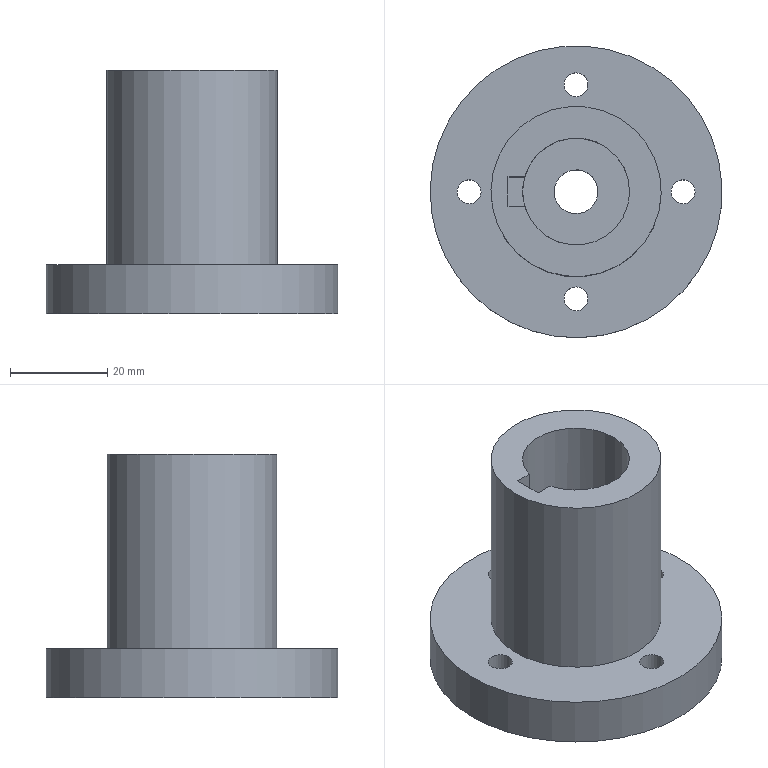Part | STEP file | SN10_010_004_EIXO | 1 solid | 18 faces | box 60 x 60 x 50 mm | volume 51834 mm3 | cylinder 9 | plane 9 | commonest cylinder face diameters 4.917 x4 9 x1 15 x1 22 x1 35 x1 60 x1
STEP:
#1=CARTESIAN_POINT('',(0.,0.,0.));
#2=DIRECTION('',(0.,0.,1.));
#3=DIRECTION('',(1.,0.,0.));
#4=AXIS2_PLACEMENT_3D('',#1,#2,#3);
#5=CARTESIAN_POINT('',(315.286,-1.179,392.5));
#6=VERTEX_POINT('',#5);
#7=CARTESIAN_POINT('',(313.129,0.,392.5));
#8=DIRECTION('',(0.,0.,-1.));
#9=DIRECTION('',(1.,0.,0.));
#10=AXIS2_PLACEMENT_3D('',#7,#8,#9);
#11=CIRCLE('',#10,2.458);
#12=CARTESIAN_POINT('',(313.129,0.,392.4));
#13=DIRECTION('',(0.,0.,-1.));
#14=DIRECTION('',(0.8776,-0.4794,0.));
#15=AXIS2_PLACEMENT_3D('',#12,#13,#14);
#16=CYLINDRICAL_SURFACE('',#15,2.458);
#17=CARTESIAN_POINT('',(-0.5,-0.1));
#18=DIRECTION('',(1.,0.));
#19=VECTOR('',#18,1.);
#20=LINE('',#17,#19);
#21=(GEOMETRIC_REPRESENTATION_CONTEXT(2)PARAMETRIC_REPRESENTATION_CONTEXT()REPRESENTATION_CONTEXT('',''));
#22=DEFINITIONAL_REPRESENTATION('',(#20),#21);
#23=PCURVE('',#16,#22);
#24=CARTESIAN_POINT('',(291.129,17.5,392.5));
#25=DIRECTION('',(0.,0.,1.));
#26=DIRECTION('',(1.,0.,0.));
#27=AXIS2_PLACEMENT_3D('',#24,#25,#26);
#28=PLANE('',#27);
#29=CARTESIAN_POINT('',(24.459,-17.5));
#30=CARTESIAN_POINT('',(24.459,-21.758));
#31=CARTESIAN_POINT('',(20.771,-19.629));
#32=CARTESIAN_POINT('',(17.083,-17.5));
#33=CARTESIAN_POINT('',(20.771,-15.371));
#34=CARTESIAN_POINT('',(24.459,-13.242));
#35=CARTESIAN_POINT('',(24.459,-17.5));
#36=(BOUNDED_CURVE()B_SPLINE_CURVE(2,(#29,#30,#31,#32,#33,#34,#35),.UNSPECIFIED.,.T.,.F.)B_SPLINE_CURVE_WITH_KNOTS((1,2,2,2,2,1),(-2.094,0.,2.094,4.189,6.283,8.378),.UNSPECIFIED.)CURVE()GEOMETRIC_REPRESENTATION_ITEM()RATIONAL_B_SPLINE_CURVE((1.,0.5,1.,0.5,1.,0.5,1.))REPRESENTATION_ITEM(''));
#37=(GEOMETRIC_REPRESENTATION_CONTEXT(2)PARAMETRIC_REPRESENTATION_CONTEXT()REPRESENTATION_CONTEXT('',''));
#38=DEFINITIONAL_REPRESENTATION('',(#36),#37);
#39=PCURVE('',#28,#38);
#40=SURFACE_CURVE('',#11,(#23,#39),.PCURVE_S1.);
#41=EDGE_CURVE('',#6,#6,#40,.T.);
#42=ORIENTED_EDGE('',*,*,#41,.T.);
#43=CARTESIAN_POINT('',(315.286,-1.179,382.5));
#44=VERTEX_POINT('',#43);
#45=CARTESIAN_POINT('',(315.286,-1.179,392.5));
#46=CARTESIAN_POINT('',(315.286,-1.179,382.5));
#47=B_SPLINE_CURVE_WITH_KNOTS('',1,(#45,#46),.UNSPECIFIED.,.F.,.F.,(2,2),(-0.1,9.9),.PIECEWISE_BEZIER_KNOTS.);
#48=CARTESIAN_POINT('',(6.283,0.));
#49=DIRECTION('',(0.,1.));
#50=VECTOR('',#49,1.);
#51=LINE('',#48,#50);
#52=(GEOMETRIC_REPRESENTATION_CONTEXT(2)PARAMETRIC_REPRESENTATION_CONTEXT()REPRESENTATION_CONTEXT('',''));
#53=DEFINITIONAL_REPRESENTATION('',(#51),#52);
#54=PCURVE('',#16,#53);
#55=CARTESIAN_POINT('',(0.,0.));
#56=DIRECTION('',(0.,1.));
#57=VECTOR('',#56,1.);
#58=LINE('',#55,#57);
#59=(GEOMETRIC_REPRESENTATION_CONTEXT(2)PARAMETRIC_REPRESENTATION_CONTEXT()REPRESENTATION_CONTEXT('',''));
#60=DEFINITIONAL_REPRESENTATION('',(#58),#59);
#61=PCURVE('',#16,#60);
#62=SEAM_CURVE('',#47,(#54,#61),.PCURVE_S1.);
#63=EDGE_CURVE('',#6,#44,#62,.T.);
#64=ORIENTED_EDGE('',*,*,#63,.T.);
#65=CARTESIAN_POINT('',(313.129,0.,382.5));
#66=DIRECTION('',(0.,0.,-1.));
#67=DIRECTION('',(1.,0.,0.));
#68=AXIS2_PLACEMENT_3D('',#65,#66,#67);
#69=CIRCLE('',#68,2.458);
#70=CARTESIAN_POINT('',(-0.5,9.9));
#71=DIRECTION('',(1.,0.));
#72=VECTOR('',#71,1.);
#73=LINE('',#70,#72);
#74=(GEOMETRIC_REPRESENTATION_CONTEXT(2)PARAMETRIC_REPRESENTATION_CONTEXT()REPRESENTATION_CONTEXT('',''));
#75=DEFINITIONAL_REPRESENTATION('',(#73),#74);
#76=PCURVE('',#16,#75);
#77=CARTESIAN_POINT('',(291.129,30.,382.5));
#78=DIRECTION('',(0.,0.,1.));
#79=DIRECTION('',(1.,0.,0.));
#80=AXIS2_PLACEMENT_3D('',#77,#78,#79);
#81=PLANE('',#80);
#82=CARTESIAN_POINT('',(24.459,-30.));
#83=CARTESIAN_POINT('',(24.459,-34.258));
#84=CARTESIAN_POINT('',(20.771,-32.129));
#85=CARTESIAN_POINT('',(17.083,-30.));
#86=CARTESIAN_POINT('',(20.771,-27.871));
#87=CARTESIAN_POINT('',(24.459,-25.742));
#88=CARTESIAN_POINT('',(24.459,-30.));
#89=(BOUNDED_CURVE()B_SPLINE_CURVE(2,(#82,#83,#84,#85,#86,#87,#88),.UNSPECIFIED.,.T.,.F.)B_SPLINE_CURVE_WITH_KNOTS((1,2,2,2,2,1),(-2.094,0.,2.094,4.189,6.283,8.378),.UNSPECIFIED.)CURVE()GEOMETRIC_REPRESENTATION_ITEM()RATIONAL_B_SPLINE_CURVE((1.,0.5,1.,0.5,1.,0.5,1.))REPRESENTATION_ITEM(''));
#90=(GEOMETRIC_REPRESENTATION_CONTEXT(2)PARAMETRIC_REPRESENTATION_CONTEXT()REPRESENTATION_CONTEXT('',''));
#91=DEFINITIONAL_REPRESENTATION('',(#89),#90);
#92=PCURVE('',#81,#91);
#93=SURFACE_CURVE('',#69,(#76,#92),.PCURVE_S1.);
#94=EDGE_CURVE('',#44,#44,#93,.T.);
#95=ORIENTED_EDGE('',*,*,#94,.F.);
#96=ORIENTED_EDGE('',*,*,#63,.F.);
#97=EDGE_LOOP('',(#42,#64,#95,#96));
#98=FACE_BOUND('',#97,.F.);
#99=ADVANCED_FACE('',(#98),#16,.F.);
#100=CARTESIAN_POINT('',(305.512,-26.327,382.5));
#101=VERTEX_POINT('',#100);
#102=CARTESIAN_POINT('',(291.129,0.,382.5));
#103=DIRECTION('',(0.,0.,1.));
#104=DIRECTION('',(1.,0.,0.));
#105=AXIS2_PLACEMENT_3D('',#102,#103,#104);
#106=CIRCLE('',#105,30.);
#107=CARTESIAN_POINT('',(291.129,0.,407.5));
#108=DIRECTION('',(0.,0.,1.));
#109=DIRECTION('',(-0.4794,0.8776,0.));
#110=AXIS2_PLACEMENT_3D('',#107,#108,#109);
#111=CYLINDRICAL_SURFACE('',#110,30.);
#112=CARTESIAN_POINT('',(-2.071,-25.));
#113=DIRECTION('',(1.,0.));
#114=VECTOR('',#113,1.);
#115=LINE('',#112,#114);
#116=(GEOMETRIC_REPRESENTATION_CONTEXT(2)PARAMETRIC_REPRESENTATION_CONTEXT()REPRESENTATION_CONTEXT('',''));
#117=DEFINITIONAL_REPRESENTATION('',(#115),#116);
#118=PCURVE('',#111,#117);
#119=CARTESIAN_POINT('',(0.,-30.));
#120=DIRECTION('',(1.,0.));
#121=AXIS2_PLACEMENT_2D('',#119,#120);
#122=CIRCLE('',#121,30.);
#123=(GEOMETRIC_REPRESENTATION_CONTEXT(2)PARAMETRIC_REPRESENTATION_CONTEXT()REPRESENTATION_CONTEXT('',''));
#124=DEFINITIONAL_REPRESENTATION('',(#122),#123);
#125=PCURVE('',#81,#124);
#126=SURFACE_CURVE('',#106,(#118,#125),.PCURVE_S1.);
#127=EDGE_CURVE('',#101,#101,#126,.T.);
#128=ORIENTED_EDGE('',*,*,#127,.T.);
#129=CARTESIAN_POINT('',(305.512,-26.327,392.5));
#130=VERTEX_POINT('',#129);
#131=CARTESIAN_POINT('',(305.512,-26.327,382.5));
#132=CARTESIAN_POINT('',(305.512,-26.327,392.5));
#133=B_SPLINE_CURVE_WITH_KNOTS('',1,(#131,#132),.UNSPECIFIED.,.F.,.F.,(2,2),(-25.,-15.),.PIECEWISE_BEZIER_KNOTS.);
#134=CARTESIAN_POINT('',(9.425,0.));
#135=DIRECTION('',(0.,1.));
#136=VECTOR('',#135,1.);
#137=LINE('',#134,#136);
#138=(GEOMETRIC_REPRESENTATION_CONTEXT(2)PARAMETRIC_REPRESENTATION_CONTEXT()REPRESENTATION_CONTEXT('',''));
#139=DEFINITIONAL_REPRESENTATION('',(#137),#138);
#140=PCURVE('',#111,#139);
#141=CARTESIAN_POINT('',(3.142,0.));
#142=DIRECTION('',(0.,1.));
#143=VECTOR('',#142,1.);
#144=LINE('',#141,#143);
#145=(GEOMETRIC_REPRESENTATION_CONTEXT(2)PARAMETRIC_REPRESENTATION_CONTEXT()REPRESENTATION_CONTEXT('',''));
#146=DEFINITIONAL_REPRESENTATION('',(#144),#145);
#147=PCURVE('',#111,#146);
#148=SEAM_CURVE('',#133,(#140,#147),.PCURVE_S1.);
#149=EDGE_CURVE('',#101,#130,#148,.T.);
#150=ORIENTED_EDGE('',*,*,#149,.T.);
#151=CARTESIAN_POINT('',(291.129,0.,392.5));
#152=DIRECTION('',(0.,0.,1.));
#153=DIRECTION('',(1.,0.,0.));
#154=AXIS2_PLACEMENT_3D('',#151,#152,#153);
#155=CIRCLE('',#154,30.);
#156=CARTESIAN_POINT('',(-2.071,-15.));
#157=DIRECTION('',(1.,0.));
#158=VECTOR('',#157,1.);
#159=LINE('',#156,#158);
#160=(GEOMETRIC_REPRESENTATION_CONTEXT(2)PARAMETRIC_REPRESENTATION_CONTEXT()REPRESENTATION_CONTEXT('',''));
#161=DEFINITIONAL_REPRESENTATION('',(#159),#160);
#162=PCURVE('',#111,#161);
#163=CARTESIAN_POINT('',(0.,-17.5));
#164=DIRECTION('',(1.,0.));
#165=AXIS2_PLACEMENT_2D('',#163,#164);
#166=CIRCLE('',#165,30.);
#167=(GEOMETRIC_REPRESENTATION_CONTEXT(2)PARAMETRIC_REPRESENTATION_CONTEXT()REPRESENTATION_CONTEXT('',''));
#168=DEFINITIONAL_REPRESENTATION('',(#166),#167);
#169=PCURVE('',#28,#168);
#170=SURFACE_CURVE('',#155,(#162,#169),.PCURVE_S1.);
#171=EDGE_CURVE('',#130,#130,#170,.T.);
#172=ORIENTED_EDGE('',*,*,#171,.F.);
#173=ORIENTED_EDGE('',*,*,#149,.F.);
#174=EDGE_LOOP('',(#128,#150,#172,#173));
#175=FACE_BOUND('',#174,.T.);
#176=ADVANCED_FACE('',(#175),#111,.T.);
#177=CARTESIAN_POINT('',(284.547,-3.596,382.5));
#178=VERTEX_POINT('',#177);
#179=CARTESIAN_POINT('',(291.129,0.,382.5));
#180=DIRECTION('',(0.,0.,1.));
#181=DIRECTION('',(1.,0.,0.));
#182=AXIS2_PLACEMENT_3D('',#179,#180,#181);
#183=CIRCLE('',#182,7.5);
#184=CARTESIAN_POINT('',(291.129,0.,382.6));
#185=DIRECTION('',(0.,0.,1.));
#186=DIRECTION('',(0.8776,0.4794,0.));
#187=AXIS2_PLACEMENT_3D('',#184,#185,#186);
#188=CYLINDRICAL_SURFACE('',#187,7.5);
#189=CARTESIAN_POINT('',(-0.5,-0.1));
#190=DIRECTION('',(1.,0.));
#191=VECTOR('',#190,1.);
#192=LINE('',#189,#191);
#193=(GEOMETRIC_REPRESENTATION_CONTEXT(2)PARAMETRIC_REPRESENTATION_CONTEXT()REPRESENTATION_CONTEXT('',''));
#194=DEFINITIONAL_REPRESENTATION('',(#192),#193);
#195=PCURVE('',#188,#194);
#196=CARTESIAN_POINT('',(0.,-30.));
#197=DIRECTION('',(1.,0.));
#198=AXIS2_PLACEMENT_2D('',#196,#197);
#199=CIRCLE('',#198,7.5);
#200=(GEOMETRIC_REPRESENTATION_CONTEXT(2)PARAMETRIC_REPRESENTATION_CONTEXT()REPRESENTATION_CONTEXT('',''));
#201=DEFINITIONAL_REPRESENTATION('',(#199),#200);
#202=PCURVE('',#81,#201);
#203=SURFACE_CURVE('',#183,(#195,#202),.PCURVE_S1.);
#204=EDGE_CURVE('',#178,#178,#203,.T.);
#205=ORIENTED_EDGE('',*,*,#204,.T.);
#206=CARTESIAN_POINT('',(284.547,-3.596,391.5));
#207=VERTEX_POINT('',#206);
#208=CARTESIAN_POINT('',(284.547,-3.596,382.5));
#209=CARTESIAN_POINT('',(284.547,-3.596,391.5));
#210=B_SPLINE_CURVE_WITH_KNOTS('',1,(#208,#209),.UNSPECIFIED.,.F.,.F.,(2,2),(-0.1,8.9),.PIECEWISE_BEZIER_KNOTS.);
#211=CARTESIAN_POINT('',(9.425,0.));
#212=DIRECTION('',(0.,1.));
#213=VECTOR('',#212,1.);
#214=LINE('',#211,#213);
#215=(GEOMETRIC_REPRESENTATION_CONTEXT(2)PARAMETRIC_REPRESENTATION_CONTEXT()REPRESENTATION_CONTEXT('',''));
#216=DEFINITIONAL_REPRESENTATION('',(#214),#215);
#217=PCURVE('',#188,#216);
#218=CARTESIAN_POINT('',(3.142,0.));
#219=DIRECTION('',(0.,1.));
#220=VECTOR('',#219,1.);
#221=LINE('',#218,#220);
#222=(GEOMETRIC_REPRESENTATION_CONTEXT(2)PARAMETRIC_REPRESENTATION_CONTEXT()REPRESENTATION_CONTEXT('',''));
#223=DEFINITIONAL_REPRESENTATION('',(#221),#222);
#224=PCURVE('',#188,#223);
#225=SEAM_CURVE('',#210,(#217,#224),.PCURVE_S1.);
#226=EDGE_CURVE('',#178,#207,#225,.T.);
#227=ORIENTED_EDGE('',*,*,#226,.T.);
#228=CARTESIAN_POINT('',(291.129,0.,391.5));
#229=DIRECTION('',(0.,0.,1.));
#230=DIRECTION('',(1.,0.,0.));
#231=AXIS2_PLACEMENT_3D('',#228,#229,#230);
#232=CIRCLE('',#231,7.5);
#233=CARTESIAN_POINT('',(-0.5,8.9));
#234=DIRECTION('',(1.,0.));
#235=VECTOR('',#234,1.);
#236=LINE('',#233,#235);
#237=(GEOMETRIC_REPRESENTATION_CONTEXT(2)PARAMETRIC_REPRESENTATION_CONTEXT()REPRESENTATION_CONTEXT('',''));
#238=DEFINITIONAL_REPRESENTATION('',(#236),#237);
#239=PCURVE('',#188,#238);
#240=CARTESIAN_POINT('',(295.629,0.,391.5));
#241=DIRECTION('',(0.,0.,1.));
#242=DIRECTION('',(1.,0.,0.));
#243=AXIS2_PLACEMENT_3D('',#240,#241,#242);
#244=PLANE('',#243);
#245=CARTESIAN_POINT('',(-4.5,0.));
#246=DIRECTION('',(1.,0.));
#247=AXIS2_PLACEMENT_2D('',#245,#246);
#248=CIRCLE('',#247,7.5);
#249=(GEOMETRIC_REPRESENTATION_CONTEXT(2)PARAMETRIC_REPRESENTATION_CONTEXT()REPRESENTATION_CONTEXT('',''));
#250=DEFINITIONAL_REPRESENTATION('',(#248),#249);
#251=PCURVE('',#244,#250);
#252=SURFACE_CURVE('',#232,(#239,#251),.PCURVE_S1.);
#253=EDGE_CURVE('',#207,#207,#252,.T.);
#254=ORIENTED_EDGE('',*,*,#253,.F.);
#255=ORIENTED_EDGE('',*,*,#226,.F.);
#256=EDGE_LOOP('',(#205,#227,#254,#255));
#257=FACE_BOUND('',#256,.F.);
#258=ADVANCED_FACE('',(#257),#188,.F.);
#259=ORIENTED_EDGE('',*,*,#253,.F.);
#260=EDGE_LOOP('',(#259));
#261=FACE_BOUND('',#260,.T.);
#262=CARTESIAN_POINT('',(295.078,2.157,391.5));
#263=VERTEX_POINT('',#262);
#264=CARTESIAN_POINT('',(291.129,0.,391.5));
#265=DIRECTION('',(0.,0.,1.));
#266=DIRECTION('',(1.,0.,0.));
#267=AXIS2_PLACEMENT_3D('',#264,#265,#266);
#268=CIRCLE('',#267,4.5);
#269=CARTESIAN_POINT('',(-4.5,0.));
#270=DIRECTION('',(1.,0.));
#271=AXIS2_PLACEMENT_2D('',#269,#270);
#272=CIRCLE('',#271,4.5);
#273=(GEOMETRIC_REPRESENTATION_CONTEXT(2)PARAMETRIC_REPRESENTATION_CONTEXT()REPRESENTATION_CONTEXT('',''));
#274=DEFINITIONAL_REPRESENTATION('',(#272),#273);
#275=PCURVE('',#244,#274);
#276=CARTESIAN_POINT('',(291.129,0.,382.6));
#277=DIRECTION('',(0.,0.,1.));
#278=DIRECTION('',(0.8776,0.4794,0.));
#279=AXIS2_PLACEMENT_3D('',#276,#277,#278);
#280=CYLINDRICAL_SURFACE('',#279,4.5);
#281=CARTESIAN_POINT('',(-0.5,8.9));
#282=DIRECTION('',(1.,0.));
#283=VECTOR('',#282,1.);
#284=LINE('',#281,#283);
#285=(GEOMETRIC_REPRESENTATION_CONTEXT(2)PARAMETRIC_REPRESENTATION_CONTEXT()REPRESENTATION_CONTEXT('',''));
#286=DEFINITIONAL_REPRESENTATION('',(#284),#285);
#287=PCURVE('',#280,#286);
#288=SURFACE_CURVE('',#268,(#275,#287),.PCURVE_S1.);
#289=EDGE_CURVE('',#263,#263,#288,.T.);
#290=ORIENTED_EDGE('',*,*,#289,.T.);
#291=EDGE_LOOP('',(#290));
#292=FACE_BOUND('',#291,.T.);
#293=ADVANCED_FACE('',(#261,#292),#244,.F.);
#294=CARTESIAN_POINT('',(295.078,2.157,402.5));
#295=VERTEX_POINT('',#294);
#296=CARTESIAN_POINT('',(291.129,0.,402.5));
#297=DIRECTION('',(0.,0.,1.));
#298=DIRECTION('',(1.,0.,0.));
#299=AXIS2_PLACEMENT_3D('',#296,#297,#298);
#300=CIRCLE('',#299,4.5);
#301=CARTESIAN_POINT('',(-0.5,19.9));
#302=DIRECTION('',(1.,0.));
#303=VECTOR('',#302,1.);
#304=LINE('',#301,#303);
#305=(GEOMETRIC_REPRESENTATION_CONTEXT(2)PARAMETRIC_REPRESENTATION_CONTEXT()REPRESENTATION_CONTEXT('',''));
#306=DEFINITIONAL_REPRESENTATION('',(#304),#305);
#307=PCURVE('',#280,#306);
#308=CARTESIAN_POINT('',(291.129,0.,402.5));
#309=DIRECTION('',(0.,0.,-1.));
#310=DIRECTION('',(-1.,0.,0.));
#311=AXIS2_PLACEMENT_3D('',#308,#309,#310);
#312=PLANE('',#311);
#313=CARTESIAN_POINT('',(-4.5,0.));
#314=CARTESIAN_POINT('',(-4.5,7.794));
#315=CARTESIAN_POINT('',(2.25,3.897));
#316=CARTESIAN_POINT('',(9.,0.));
#317=CARTESIAN_POINT('',(2.25,-3.897));
#318=CARTESIAN_POINT('',(-4.5,-7.794));
#319=CARTESIAN_POINT('',(-4.5,0.));
#320=(BOUNDED_CURVE()B_SPLINE_CURVE(2,(#313,#314,#315,#316,#317,#318,#319),.UNSPECIFIED.,.T.,.F.)B_SPLINE_CURVE_WITH_KNOTS((1,2,2,2,2,1),(-2.094,0.,2.094,4.189,6.283,8.378),.UNSPECIFIED.)CURVE()GEOMETRIC_REPRESENTATION_ITEM()RATIONAL_B_SPLINE_CURVE((1.,0.5,1.,0.5,1.,0.5,1.))REPRESENTATION_ITEM(''));
#321=(GEOMETRIC_REPRESENTATION_CONTEXT(2)PARAMETRIC_REPRESENTATION_CONTEXT()REPRESENTATION_CONTEXT('',''));
#322=DEFINITIONAL_REPRESENTATION('',(#320),#321);
#323=PCURVE('',#312,#322);
#324=SURFACE_CURVE('',#300,(#307,#323),.PCURVE_S1.);
#325=EDGE_CURVE('',#295,#295,#324,.T.);
#326=ORIENTED_EDGE('',*,*,#325,.F.);
#327=CARTESIAN_POINT('',(295.078,2.157,391.5));
#328=CARTESIAN_POINT('',(295.078,2.157,402.5));
#329=B_SPLINE_CURVE_WITH_KNOTS('',1,(#327,#328),.UNSPECIFIED.,.F.,.F.,(2,2),(8.9,19.9),.PIECEWISE_BEZIER_KNOTS.);
#330=CARTESIAN_POINT('',(0.,0.));
#331=DIRECTION('',(0.,1.));
#332=VECTOR('',#331,1.);
#333=LINE('',#330,#332);
#334=(GEOMETRIC_REPRESENTATION_CONTEXT(2)PARAMETRIC_REPRESENTATION_CONTEXT()REPRESENTATION_CONTEXT('',''));
#335=DEFINITIONAL_REPRESENTATION('',(#333),#334);
#336=PCURVE('',#280,#335);
#337=CARTESIAN_POINT('',(6.283,0.));
#338=DIRECTION('',(0.,1.));
#339=VECTOR('',#338,1.);
#340=LINE('',#337,#339);
#341=(GEOMETRIC_REPRESENTATION_CONTEXT(2)PARAMETRIC_REPRESENTATION_CONTEXT()REPRESENTATION_CONTEXT('',''));
#342=DEFINITIONAL_REPRESENTATION('',(#340),#341);
#343=PCURVE('',#280,#342);
#344=SEAM_CURVE('',#329,(#336,#343),.PCURVE_S1.);
#345=EDGE_CURVE('',#263,#295,#344,.T.);
#346=ORIENTED_EDGE('',*,*,#345,.F.);
#347=ORIENTED_EDGE('',*,*,#289,.T.);
#348=ORIENTED_EDGE('',*,*,#345,.T.);
#349=EDGE_LOOP('',(#326,#346,#347,#348));
#350=FACE_BOUND('',#349,.F.);
#351=ADVANCED_FACE('',(#350),#280,.F.);
#352=CARTESIAN_POINT('',(280.546,-3.,432.5));
#353=VERTEX_POINT('',#352);
#354=CARTESIAN_POINT('',(280.546,-3.,407.5));
#355=VERTEX_POINT('',#354);
#356=CARTESIAN_POINT('',(280.546,-3.,432.5));
#357=DIRECTION('',(0.,0.,-1.));
#358=VECTOR('',#357,1.);
#359=LINE('',#356,#358);
#360=CARTESIAN_POINT('',(291.129,0.,432.4));
#361=DIRECTION('',(0.,0.,-1.));
#362=DIRECTION('',(0.8776,-0.4794,0.));
#363=AXIS2_PLACEMENT_3D('',#360,#361,#362);
#364=CYLINDRICAL_SURFACE('',#363,11.);
#365=CARTESIAN_POINT('',(2.365,-0.1));
#366=DIRECTION('',(0.,1.));
#367=VECTOR('',#366,1.);
#368=LINE('',#365,#367);
#369=(GEOMETRIC_REPRESENTATION_CONTEXT(2)PARAMETRIC_REPRESENTATION_CONTEXT()REPRESENTATION_CONTEXT('',''));
#370=DEFINITIONAL_REPRESENTATION('',(#368),#369);
#371=PCURVE('',#364,#370);
#372=CARTESIAN_POINT('',(277.129,-3.,432.5));
#373=DIRECTION('',(0.,1.,0.));
#374=DIRECTION('',(0.,0.,1.));
#375=AXIS2_PLACEMENT_3D('',#372,#373,#374);
#376=PLANE('',#375);
#377=CARTESIAN_POINT('',(0.,3.417));
#378=DIRECTION('',(-1.,0.));
#379=VECTOR('',#378,1.);
#380=LINE('',#377,#379);
#381=(GEOMETRIC_REPRESENTATION_CONTEXT(2)PARAMETRIC_REPRESENTATION_CONTEXT()REPRESENTATION_CONTEXT('',''));
#382=DEFINITIONAL_REPRESENTATION('',(#380),#381);
#383=PCURVE('',#376,#382);
#384=SURFACE_CURVE('',#359,(#371,#383),.PCURVE_S1.);
#385=EDGE_CURVE('',#353,#355,#384,.T.);
#386=ORIENTED_EDGE('',*,*,#385,.T.);
#387=CARTESIAN_POINT('',(280.546,3.,407.5));
#388=VERTEX_POINT('',#387);
#389=CARTESIAN_POINT('',(291.129,0.,407.5));
#390=DIRECTION('',(0.,0.,-1.));
#391=DIRECTION('',(1.,0.,0.));
#392=AXIS2_PLACEMENT_3D('',#389,#390,#391);
#393=CIRCLE('',#392,11.);
#394=CARTESIAN_POINT('',(-0.5,24.9));
#395=DIRECTION('',(1.,0.));
#396=VECTOR('',#395,1.);
#397=LINE('',#394,#396);
#398=(GEOMETRIC_REPRESENTATION_CONTEXT(2)PARAMETRIC_REPRESENTATION_CONTEXT()REPRESENTATION_CONTEXT('',''));
#399=DEFINITIONAL_REPRESENTATION('',(#397),#398);
#400=PCURVE('',#364,#399);
#401=CARTESIAN_POINT('',(0.,0.,407.5));
#402=DIRECTION('',(0.,0.,1.));
#403=DIRECTION('',(1.,0.,0.));
#404=AXIS2_PLACEMENT_3D('',#401,#402,#403);
#405=PLANE('',#404);
#406=CARTESIAN_POINT('',(302.129,0.));
#407=CARTESIAN_POINT('',(302.129,-19.053));
#408=CARTESIAN_POINT('',(285.629,-9.526));
#409=CARTESIAN_POINT('',(269.129,0.));
#410=CARTESIAN_POINT('',(285.629,9.526));
#411=CARTESIAN_POINT('',(302.129,19.053));
#412=CARTESIAN_POINT('',(302.129,0.));
#413=(BOUNDED_CURVE()B_SPLINE_CURVE(2,(#406,#407,#408,#409,#410,#411,#412),.UNSPECIFIED.,.T.,.F.)B_SPLINE_CURVE_WITH_KNOTS((1,2,2,2,2,1),(-2.094,0.,2.094,4.189,6.283,8.378),.UNSPECIFIED.)CURVE()GEOMETRIC_REPRESENTATION_ITEM()RATIONAL_B_SPLINE_CURVE((1.,0.5,1.,0.5,1.,0.5,1.))REPRESENTATION_ITEM(''));
#414=(GEOMETRIC_REPRESENTATION_CONTEXT(2)PARAMETRIC_REPRESENTATION_CONTEXT()REPRESENTATION_CONTEXT('',''));
#415=DEFINITIONAL_REPRESENTATION('',(#413),#414);
#416=PCURVE('',#405,#415);
#417=SURFACE_CURVE('',#393,(#400,#416),.PCURVE_S1.);
#418=EDGE_CURVE('',#355,#388,#417,.T.);
#419=ORIENTED_EDGE('',*,*,#418,.T.);
#420=CARTESIAN_POINT('',(280.546,3.,432.5));
#421=VERTEX_POINT('',#420);
#422=CARTESIAN_POINT('',(280.546,3.,432.5));
#423=DIRECTION('',(0.,0.,-1.));
#424=VECTOR('',#423,1.);
#425=LINE('',#422,#424);
#426=CARTESIAN_POINT('',(2.918,-0.1));
#427=DIRECTION('',(0.,1.));
#428=VECTOR('',#427,1.);
#429=LINE('',#426,#428);
#430=(GEOMETRIC_REPRESENTATION_CONTEXT(2)PARAMETRIC_REPRESENTATION_CONTEXT()REPRESENTATION_CONTEXT('',''));
#431=DEFINITIONAL_REPRESENTATION('',(#429),#430);
#432=PCURVE('',#364,#431);
#433=CARTESIAN_POINT('',(280.546,3.,432.5));
#434=DIRECTION('',(0.,-1.,0.));
#435=DIRECTION('',(0.,0.,-1.));
#436=AXIS2_PLACEMENT_3D('',#433,#434,#435);
#437=PLANE('',#436);
#438=CARTESIAN_POINT('',(0.,0.));
#439=DIRECTION('',(1.,0.));
#440=VECTOR('',#439,1.);
#441=LINE('',#438,#440);
#442=(GEOMETRIC_REPRESENTATION_CONTEXT(2)PARAMETRIC_REPRESENTATION_CONTEXT()REPRESENTATION_CONTEXT('',''));
#443=DEFINITIONAL_REPRESENTATION('',(#441),#442);
#444=PCURVE('',#437,#443);
#445=SURFACE_CURVE('',#425,(#432,#444),.PCURVE_S1.);
#446=EDGE_CURVE('',#421,#388,#445,.T.);
#447=ORIENTED_EDGE('',*,*,#446,.F.);
#448=CARTESIAN_POINT('',(300.782,-5.274,432.5));
#449=VERTEX_POINT('',#448);
#450=CARTESIAN_POINT('',(291.129,0.,432.5));
#451=DIRECTION('',(0.,0.,-1.));
#452=DIRECTION('',(1.,0.,0.));
#453=AXIS2_PLACEMENT_3D('',#450,#451,#452);
#454=CIRCLE('',#453,11.);
#455=CARTESIAN_POINT('',(-0.5,-0.1));
#456=DIRECTION('',(1.,0.));
#457=VECTOR('',#456,1.);
#458=LINE('',#455,#457);
#459=(GEOMETRIC_REPRESENTATION_CONTEXT(2)PARAMETRIC_REPRESENTATION_CONTEXT()REPRESENTATION_CONTEXT('',''));
#460=DEFINITIONAL_REPRESENTATION('',(#458),#459);
#461=PCURVE('',#364,#460);
#462=CARTESIAN_POINT('',(291.129,0.,432.5));
#463=DIRECTION('',(0.,0.,1.));
#464=DIRECTION('',(1.,0.,0.));
#465=AXIS2_PLACEMENT_3D('',#462,#463,#464);
#466=PLANE('',#465);
#467=CARTESIAN_POINT('',(11.,0.));
#468=CARTESIAN_POINT('',(11.,-19.053));
#469=CARTESIAN_POINT('',(-5.5,-9.526));
#470=CARTESIAN_POINT('',(-22.,0.));
#471=CARTESIAN_POINT('',(-5.5,9.526));
#472=CARTESIAN_POINT('',(11.,19.053));
#473=CARTESIAN_POINT('',(11.,0.));
#474=(BOUNDED_CURVE()B_SPLINE_CURVE(2,(#467,#468,#469,#470,#471,#472,#473),.UNSPECIFIED.,.T.,.F.)B_SPLINE_CURVE_WITH_KNOTS((1,2,2,2,2,1),(-2.094,0.,2.094,4.189,6.283,8.378),.UNSPECIFIED.)CURVE()GEOMETRIC_REPRESENTATION_ITEM()RATIONAL_B_SPLINE_CURVE((1.,0.5,1.,0.5,1.,0.5,1.))REPRESENTATION_ITEM(''));
#475=(GEOMETRIC_REPRESENTATION_CONTEXT(2)PARAMETRIC_REPRESENTATION_CONTEXT()REPRESENTATION_CONTEXT('',''));
#476=DEFINITIONAL_REPRESENTATION('',(#474),#475);
#477=PCURVE('',#466,#476);
#478=SURFACE_CURVE('',#454,(#461,#477),.PCURVE_S1.);
#479=EDGE_CURVE('',#421,#449,#478,.T.);
#480=ORIENTED_EDGE('',*,*,#479,.T.);
#481=CARTESIAN_POINT('',(300.782,-5.274,402.5));
#482=VERTEX_POINT('',#481);
#483=CARTESIAN_POINT('',(300.782,-5.274,432.5));
#484=CARTESIAN_POINT('',(300.782,-5.274,402.5));
#485=B_SPLINE_CURVE_WITH_KNOTS('',1,(#483,#484),.UNSPECIFIED.,.F.,.F.,(2,2),(-0.1,29.9),.PIECEWISE_BEZIER_KNOTS.);
#486=CARTESIAN_POINT('',(6.283,0.));
#487=DIRECTION('',(0.,1.));
#488=VECTOR('',#487,1.);
#489=LINE('',#486,#488);
#490=(GEOMETRIC_REPRESENTATION_CONTEXT(2)PARAMETRIC_REPRESENTATION_CONTEXT()REPRESENTATION_CONTEXT('',''));
#491=DEFINITIONAL_REPRESENTATION('',(#489),#490);
#492=PCURVE('',#364,#491);
#493=CARTESIAN_POINT('',(0.,0.));
#494=DIRECTION('',(0.,1.));
#495=VECTOR('',#494,1.);
#496=LINE('',#493,#495);
#497=(GEOMETRIC_REPRESENTATION_CONTEXT(2)PARAMETRIC_REPRESENTATION_CONTEXT()REPRESENTATION_CONTEXT('',''));
#498=DEFINITIONAL_REPRESENTATION('',(#496),#497);
#499=PCURVE('',#364,#498);
#500=SEAM_CURVE('',#485,(#492,#499),.PCURVE_S1.);
#501=EDGE_CURVE('',#449,#482,#500,.T.);
#502=ORIENTED_EDGE('',*,*,#501,.T.);
#503=CARTESIAN_POINT('',(291.129,0.,402.5));
#504=DIRECTION('',(0.,0.,-1.));
#505=DIRECTION('',(1.,0.,0.));
#506=AXIS2_PLACEMENT_3D('',#503,#504,#505);
#507=CIRCLE('',#506,11.);
#508=CARTESIAN_POINT('',(-0.5,29.9));
#509=DIRECTION('',(1.,0.));
#510=VECTOR('',#509,1.);
#511=LINE('',#508,#510);
#512=(GEOMETRIC_REPRESENTATION_CONTEXT(2)PARAMETRIC_REPRESENTATION_CONTEXT()REPRESENTATION_CONTEXT('',''));
#513=DEFINITIONAL_REPRESENTATION('',(#511),#512);
#514=PCURVE('',#364,#513);
#515=CARTESIAN_POINT('',(0.,0.));
#516=DIRECTION('',(-1.,0.));
#517=AXIS2_PLACEMENT_2D('',#515,#516);
#518=CIRCLE('',#517,11.);
#519=(GEOMETRIC_REPRESENTATION_CONTEXT(2)PARAMETRIC_REPRESENTATION_CONTEXT()REPRESENTATION_CONTEXT('',''));
#520=DEFINITIONAL_REPRESENTATION('',(#518),#519);
#521=PCURVE('',#312,#520);
#522=SURFACE_CURVE('',#507,(#514,#521),.PCURVE_S1.);
#523=EDGE_CURVE('',#482,#482,#522,.T.);
#524=ORIENTED_EDGE('',*,*,#523,.F.);
#525=ORIENTED_EDGE('',*,*,#501,.F.);
#526=CARTESIAN_POINT('',(291.129,0.,432.5));
#527=DIRECTION('',(0.,0.,-1.));
#528=DIRECTION('',(1.,0.,0.));
#529=AXIS2_PLACEMENT_3D('',#526,#527,#528);
#530=CIRCLE('',#529,11.);
#531=CARTESIAN_POINT('',(-0.5,-0.1));
#532=DIRECTION('',(1.,0.));
#533=VECTOR('',#532,1.);
#534=LINE('',#531,#533);
#535=(GEOMETRIC_REPRESENTATION_CONTEXT(2)PARAMETRIC_REPRESENTATION_CONTEXT()REPRESENTATION_CONTEXT('',''));
#536=DEFINITIONAL_REPRESENTATION('',(#534),#535);
#537=PCURVE('',#364,#536);
#538=CARTESIAN_POINT('',(11.,0.));
#539=CARTESIAN_POINT('',(11.,-19.053));
#540=CARTESIAN_POINT('',(-5.5,-9.526));
#541=CARTESIAN_POINT('',(-22.,0.));
#542=CARTESIAN_POINT('',(-5.5,9.526));
#543=CARTESIAN_POINT('',(11.,19.053));
#544=CARTESIAN_POINT('',(11.,0.));
#545=(BOUNDED_CURVE()B_SPLINE_CURVE(2,(#538,#539,#540,#541,#542,#543,#544),.UNSPECIFIED.,.T.,.F.)B_SPLINE_CURVE_WITH_KNOTS((1,2,2,2,2,1),(-2.094,0.,2.094,4.189,6.283,8.378),.UNSPECIFIED.)CURVE()GEOMETRIC_REPRESENTATION_ITEM()RATIONAL_B_SPLINE_CURVE((1.,0.5,1.,0.5,1.,0.5,1.))REPRESENTATION_ITEM(''));
#546=(GEOMETRIC_REPRESENTATION_CONTEXT(2)PARAMETRIC_REPRESENTATION_CONTEXT()REPRESENTATION_CONTEXT('',''));
#547=DEFINITIONAL_REPRESENTATION('',(#545),#546);
#548=PCURVE('',#466,#547);
#549=SURFACE_CURVE('',#530,(#537,#548),.PCURVE_S1.);
#550=EDGE_CURVE('',#449,#353,#549,.T.);
#551=ORIENTED_EDGE('',*,*,#550,.T.);
#552=EDGE_LOOP('',(#386,#419,#447,#480,#502,#524,#525,#551));
#553=FACE_BOUND('',#552,.F.);
#554=ADVANCED_FACE('',(#553),#364,.F.);
#555=ORIENTED_EDGE('',*,*,#523,.F.);
#556=EDGE_LOOP('',(#555));
#557=FACE_BOUND('',#556,.T.);
#558=ORIENTED_EDGE('',*,*,#325,.F.);
#559=EDGE_LOOP('',(#558));
#560=FACE_BOUND('',#559,.T.);
#561=ADVANCED_FACE('',(#557,#560),#312,.F.);
#562=CARTESIAN_POINT('',(299.519,-15.358,392.5));
#563=VERTEX_POINT('',#562);
#564=CARTESIAN_POINT('',(291.129,0.,392.5));
#565=DIRECTION('',(0.,0.,1.));
#566=DIRECTION('',(1.,0.,0.));
#567=AXIS2_PLACEMENT_3D('',#564,#565,#566);
#568=CIRCLE('',#567,17.5);
#569=CARTESIAN_POINT('',(291.129,0.,407.5));
#570=DIRECTION('',(0.,0.,1.));
#571=DIRECTION('',(-0.4794,0.8776,0.));
#572=AXIS2_PLACEMENT_3D('',#569,#570,#571);
#573=CYLINDRICAL_SURFACE('',#572,17.5);
#574=CARTESIAN_POINT('',(-2.071,-15.));
#575=DIRECTION('',(1.,0.));
#576=VECTOR('',#575,1.);
#577=LINE('',#574,#576);
#578=(GEOMETRIC_REPRESENTATION_CONTEXT(2)PARAMETRIC_REPRESENTATION_CONTEXT()REPRESENTATION_CONTEXT('',''));
#579=DEFINITIONAL_REPRESENTATION('',(#577),#578);
#580=PCURVE('',#573,#579);
#581=CARTESIAN_POINT('',(0.,-17.5));
#582=DIRECTION('',(1.,0.));
#583=AXIS2_PLACEMENT_2D('',#581,#582);
#584=CIRCLE('',#583,17.5);
#585=(GEOMETRIC_REPRESENTATION_CONTEXT(2)PARAMETRIC_REPRESENTATION_CONTEXT()REPRESENTATION_CONTEXT('',''));
#586=DEFINITIONAL_REPRESENTATION('',(#584),#585);
#587=PCURVE('',#28,#586);
#588=SURFACE_CURVE('',#568,(#580,#587),.PCURVE_S1.);
#589=EDGE_CURVE('',#563,#563,#588,.T.);
#590=ORIENTED_EDGE('',*,*,#589,.T.);
#591=CARTESIAN_POINT('',(299.519,-15.358,432.5));
#592=VERTEX_POINT('',#591);
#593=CARTESIAN_POINT('',(299.519,-15.358,392.5));
#594=CARTESIAN_POINT('',(299.519,-15.358,432.5));
#595=B_SPLINE_CURVE_WITH_KNOTS('',1,(#593,#594),.UNSPECIFIED.,.F.,.F.,(2,2),(-15.,25.),.PIECEWISE_BEZIER_KNOTS.);
#596=CARTESIAN_POINT('',(9.425,0.));
#597=DIRECTION('',(0.,1.));
#598=VECTOR('',#597,1.);
#599=LINE('',#596,#598);
#600=(GEOMETRIC_REPRESENTATION_CONTEXT(2)PARAMETRIC_REPRESENTATION_CONTEXT()REPRESENTATION_CONTEXT('',''));
#601=DEFINITIONAL_REPRESENTATION('',(#599),#600);
#602=PCURVE('',#573,#601);
#603=CARTESIAN_POINT('',(3.142,0.));
#604=DIRECTION('',(0.,1.));
#605=VECTOR('',#604,1.);
#606=LINE('',#603,#605);
#607=(GEOMETRIC_REPRESENTATION_CONTEXT(2)PARAMETRIC_REPRESENTATION_CONTEXT()REPRESENTATION_CONTEXT('',''));
#608=DEFINITIONAL_REPRESENTATION('',(#606),#607);
#609=PCURVE('',#573,#608);
#610=SEAM_CURVE('',#595,(#602,#609),.PCURVE_S1.);
#611=EDGE_CURVE('',#563,#592,#610,.T.);
#612=ORIENTED_EDGE('',*,*,#611,.T.);
#613=CARTESIAN_POINT('',(291.129,0.,432.5));
#614=DIRECTION('',(0.,0.,1.));
#615=DIRECTION('',(1.,0.,0.));
#616=AXIS2_PLACEMENT_3D('',#613,#614,#615);
#617=CIRCLE('',#616,17.5);
#618=CARTESIAN_POINT('',(-2.071,25.));
#619=DIRECTION('',(1.,0.));
#620=VECTOR('',#619,1.);
#621=LINE('',#618,#620);
#622=(GEOMETRIC_REPRESENTATION_CONTEXT(2)PARAMETRIC_REPRESENTATION_CONTEXT()REPRESENTATION_CONTEXT('',''));
#623=DEFINITIONAL_REPRESENTATION('',(#621),#622);
#624=PCURVE('',#573,#623);
#625=CARTESIAN_POINT('',(0.,0.));
#626=DIRECTION('',(1.,0.));
#627=AXIS2_PLACEMENT_2D('',#625,#626);
#628=CIRCLE('',#627,17.5);
#629=(GEOMETRIC_REPRESENTATION_CONTEXT(2)PARAMETRIC_REPRESENTATION_CONTEXT()REPRESENTATION_CONTEXT('',''));
#630=DEFINITIONAL_REPRESENTATION('',(#628),#629);
#631=PCURVE('',#466,#630);
#632=SURFACE_CURVE('',#617,(#624,#631),.PCURVE_S1.);
#633=EDGE_CURVE('',#592,#592,#632,.T.);
#634=ORIENTED_EDGE('',*,*,#633,.F.);
#635=ORIENTED_EDGE('',*,*,#611,.F.);
#636=EDGE_LOOP('',(#590,#612,#634,#635));
#637=FACE_BOUND('',#636,.T.);
#638=ADVANCED_FACE('',(#637),#573,.T.);
#639=ORIENTED_EDGE('',*,*,#127,.F.);
#640=EDGE_LOOP('',(#639));
#641=FACE_BOUND('',#640,.T.);
#642=ORIENTED_EDGE('',*,*,#94,.F.);
#643=EDGE_LOOP('',(#642));
#644=FACE_BOUND('',#643,.T.);
#645=ORIENTED_EDGE('',*,*,#204,.T.);
#646=EDGE_LOOP('',(#645));
#647=FACE_BOUND('',#646,.T.);
#648=CARTESIAN_POINT('',(292.308,24.158,382.5));
#649=VERTEX_POINT('',#648);
#650=CARTESIAN_POINT('',(291.129,22.,382.5));
#651=DIRECTION('',(0.,0.,1.));
#652=DIRECTION('',(1.,0.,0.));
#653=AXIS2_PLACEMENT_3D('',#650,#651,#652);
#654=CIRCLE('',#653,2.458);
#655=CARTESIAN_POINT('',(0.,-8.));
#656=DIRECTION('',(1.,0.));
#657=AXIS2_PLACEMENT_2D('',#655,#656);
#658=CIRCLE('',#657,2.458);
#659=(GEOMETRIC_REPRESENTATION_CONTEXT(2)PARAMETRIC_REPRESENTATION_CONTEXT()REPRESENTATION_CONTEXT('',''));
#660=DEFINITIONAL_REPRESENTATION('',(#658),#659);
#661=PCURVE('',#81,#660);
#662=CARTESIAN_POINT('',(291.129,22.,392.4));
#663=DIRECTION('',(0.,0.,-1.));
#664=DIRECTION('',(0.4794,0.8776,0.));
#665=AXIS2_PLACEMENT_3D('',#662,#663,#664);
#666=CYLINDRICAL_SURFACE('',#665,2.458);
#667=CARTESIAN_POINT('',(7.354,9.9));
#668=DIRECTION('',(-1.,0.));
#669=VECTOR('',#668,1.);
#670=LINE('',#667,#669);
#671=(GEOMETRIC_REPRESENTATION_CONTEXT(2)PARAMETRIC_REPRESENTATION_CONTEXT()REPRESENTATION_CONTEXT('',''));
#672=DEFINITIONAL_REPRESENTATION('',(#670),#671);
#673=PCURVE('',#666,#672);
#674=SURFACE_CURVE('',#654,(#661,#673),.PCURVE_S1.);
#675=EDGE_CURVE('',#649,#649,#674,.T.);
#676=ORIENTED_EDGE('',*,*,#675,.T.);
#677=EDGE_LOOP('',(#676));
#678=FACE_BOUND('',#677,.T.);
#679=CARTESIAN_POINT('',(266.971,1.179,382.5));
#680=VERTEX_POINT('',#679);
#681=CARTESIAN_POINT('',(269.129,0.,382.5));
#682=DIRECTION('',(0.,0.,1.));
#683=DIRECTION('',(1.,0.,0.));
#684=AXIS2_PLACEMENT_3D('',#681,#682,#683);
#685=CIRCLE('',#684,2.458);
#686=CARTESIAN_POINT('',(-22.,-30.));
#687=DIRECTION('',(1.,0.));
#688=AXIS2_PLACEMENT_2D('',#686,#687);
#689=CIRCLE('',#688,2.458);
#690=(GEOMETRIC_REPRESENTATION_CONTEXT(2)PARAMETRIC_REPRESENTATION_CONTEXT()REPRESENTATION_CONTEXT('',''));
#691=DEFINITIONAL_REPRESENTATION('',(#689),#690);
#692=PCURVE('',#81,#691);
#693=CARTESIAN_POINT('',(269.129,0.,392.4));
#694=DIRECTION('',(0.,0.,-1.));
#695=DIRECTION('',(-0.8776,0.4794,0.));
#696=AXIS2_PLACEMENT_3D('',#693,#694,#695);
#697=CYLINDRICAL_SURFACE('',#696,2.458);
#698=CARTESIAN_POINT('',(8.925,9.9));
#699=DIRECTION('',(-1.,0.));
#700=VECTOR('',#699,1.);
#701=LINE('',#698,#700);
#702=(GEOMETRIC_REPRESENTATION_CONTEXT(2)PARAMETRIC_REPRESENTATION_CONTEXT()REPRESENTATION_CONTEXT('',''));
#703=DEFINITIONAL_REPRESENTATION('',(#701),#702);
#704=PCURVE('',#697,#703);
#705=SURFACE_CURVE('',#685,(#692,#704),.PCURVE_S1.);
#706=EDGE_CURVE('',#680,#680,#705,.T.);
#707=ORIENTED_EDGE('',*,*,#706,.T.);
#708=EDGE_LOOP('',(#707));
#709=FACE_BOUND('',#708,.T.);
#710=CARTESIAN_POINT('',(289.95,-24.158,382.5));
#711=VERTEX_POINT('',#710);
#712=CARTESIAN_POINT('',(291.129,-22.,382.5));
#713=DIRECTION('',(0.,0.,1.));
#714=DIRECTION('',(1.,0.,0.));
#715=AXIS2_PLACEMENT_3D('',#712,#713,#714);
#716=CIRCLE('',#715,2.458);
#717=CARTESIAN_POINT('',(0.,-52.));
#718=DIRECTION('',(1.,0.));
#719=AXIS2_PLACEMENT_2D('',#717,#718);
#720=CIRCLE('',#719,2.458);
#721=(GEOMETRIC_REPRESENTATION_CONTEXT(2)PARAMETRIC_REPRESENTATION_CONTEXT()REPRESENTATION_CONTEXT('',''));
#722=DEFINITIONAL_REPRESENTATION('',(#720),#721);
#723=PCURVE('',#81,#722);
#724=CARTESIAN_POINT('',(291.129,-22.,392.4));
#725=DIRECTION('',(0.,0.,-1.));
#726=DIRECTION('',(-0.4794,-0.8776,0.));
#727=AXIS2_PLACEMENT_3D('',#724,#725,#726);
#728=CYLINDRICAL_SURFACE('',#727,2.458);
#729=CARTESIAN_POINT('',(10.496,9.9));
#730=DIRECTION('',(-1.,0.));
#731=VECTOR('',#730,1.);
#732=LINE('',#729,#731);
#733=(GEOMETRIC_REPRESENTATION_CONTEXT(2)PARAMETRIC_REPRESENTATION_CONTEXT()REPRESENTATION_CONTEXT('',''));
#734=DEFINITIONAL_REPRESENTATION('',(#732),#733);
#735=PCURVE('',#728,#734);
#736=SURFACE_CURVE('',#716,(#723,#735),.PCURVE_S1.);
#737=EDGE_CURVE('',#711,#711,#736,.T.);
#738=ORIENTED_EDGE('',*,*,#737,.T.);
#739=EDGE_LOOP('',(#738));
#740=FACE_BOUND('',#739,.T.);
#741=ADVANCED_FACE('',(#641,#644,#647,#678,#709,#740),#81,.F.);
#742=ORIENTED_EDGE('',*,*,#171,.T.);
#743=EDGE_LOOP('',(#742));
#744=FACE_BOUND('',#743,.T.);
#745=ORIENTED_EDGE('',*,*,#41,.T.);
#746=EDGE_LOOP('',(#745));
#747=FACE_BOUND('',#746,.T.);
#748=ORIENTED_EDGE('',*,*,#589,.F.);
#749=EDGE_LOOP('',(#748));
#750=FACE_BOUND('',#749,.T.);
#751=CARTESIAN_POINT('',(292.308,24.158,392.5));
#752=VERTEX_POINT('',#751);
#753=CARTESIAN_POINT('',(291.129,22.,392.5));
#754=DIRECTION('',(0.,0.,1.));
#755=DIRECTION('',(1.,0.,0.));
#756=AXIS2_PLACEMENT_3D('',#753,#754,#755);
#757=CIRCLE('',#756,2.458);
#758=CARTESIAN_POINT('',(0.,4.5));
#759=DIRECTION('',(1.,0.));
#760=AXIS2_PLACEMENT_2D('',#758,#759);
#761=CIRCLE('',#760,2.458);
#762=(GEOMETRIC_REPRESENTATION_CONTEXT(2)PARAMETRIC_REPRESENTATION_CONTEXT()REPRESENTATION_CONTEXT('',''));
#763=DEFINITIONAL_REPRESENTATION('',(#761),#762);
#764=PCURVE('',#28,#763);
#765=CARTESIAN_POINT('',(7.354,-0.1));
#766=DIRECTION('',(-1.,0.));
#767=VECTOR('',#766,1.);
#768=LINE('',#765,#767);
#769=(GEOMETRIC_REPRESENTATION_CONTEXT(2)PARAMETRIC_REPRESENTATION_CONTEXT()REPRESENTATION_CONTEXT('',''));
#770=DEFINITIONAL_REPRESENTATION('',(#768),#769);
#771=PCURVE('',#666,#770);
#772=SURFACE_CURVE('',#757,(#764,#771),.PCURVE_S1.);
#773=EDGE_CURVE('',#752,#752,#772,.T.);
#774=ORIENTED_EDGE('',*,*,#773,.F.);
#775=EDGE_LOOP('',(#774));
#776=FACE_BOUND('',#775,.T.);
#777=CARTESIAN_POINT('',(266.971,1.179,392.5));
#778=VERTEX_POINT('',#777);
#779=CARTESIAN_POINT('',(269.129,0.,392.5));
#780=DIRECTION('',(0.,0.,1.));
#781=DIRECTION('',(1.,0.,0.));
#782=AXIS2_PLACEMENT_3D('',#779,#780,#781);
#783=CIRCLE('',#782,2.458);
#784=CARTESIAN_POINT('',(-22.,-17.5));
#785=DIRECTION('',(1.,0.));
#786=AXIS2_PLACEMENT_2D('',#784,#785);
#787=CIRCLE('',#786,2.458);
#788=(GEOMETRIC_REPRESENTATION_CONTEXT(2)PARAMETRIC_REPRESENTATION_CONTEXT()REPRESENTATION_CONTEXT('',''));
#789=DEFINITIONAL_REPRESENTATION('',(#787),#788);
#790=PCURVE('',#28,#789);
#791=CARTESIAN_POINT('',(8.925,-0.1));
#792=DIRECTION('',(-1.,0.));
#793=VECTOR('',#792,1.);
#794=LINE('',#791,#793);
#795=(GEOMETRIC_REPRESENTATION_CONTEXT(2)PARAMETRIC_REPRESENTATION_CONTEXT()REPRESENTATION_CONTEXT('',''));
#796=DEFINITIONAL_REPRESENTATION('',(#794),#795);
#797=PCURVE('',#697,#796);
#798=SURFACE_CURVE('',#783,(#790,#797),.PCURVE_S1.);
#799=EDGE_CURVE('',#778,#778,#798,.T.);
#800=ORIENTED_EDGE('',*,*,#799,.F.);
#801=EDGE_LOOP('',(#800));
#802=FACE_BOUND('',#801,.T.);
#803=CARTESIAN_POINT('',(289.95,-24.158,392.5));
#804=VERTEX_POINT('',#803);
#805=CARTESIAN_POINT('',(291.129,-22.,392.5));
#806=DIRECTION('',(0.,0.,1.));
#807=DIRECTION('',(1.,0.,0.));
#808=AXIS2_PLACEMENT_3D('',#805,#806,#807);
#809=CIRCLE('',#808,2.458);
#810=CARTESIAN_POINT('',(0.,-39.5));
#811=DIRECTION('',(1.,0.));
#812=AXIS2_PLACEMENT_2D('',#810,#811);
#813=CIRCLE('',#812,2.458);
#814=(GEOMETRIC_REPRESENTATION_CONTEXT(2)PARAMETRIC_REPRESENTATION_CONTEXT()REPRESENTATION_CONTEXT('',''));
#815=DEFINITIONAL_REPRESENTATION('',(#813),#814);
#816=PCURVE('',#28,#815);
#817=CARTESIAN_POINT('',(10.496,-0.1));
#818=DIRECTION('',(-1.,0.));
#819=VECTOR('',#818,1.);
#820=LINE('',#817,#819);
#821=(GEOMETRIC_REPRESENTATION_CONTEXT(2)PARAMETRIC_REPRESENTATION_CONTEXT()REPRESENTATION_CONTEXT('',''));
#822=DEFINITIONAL_REPRESENTATION('',(#820),#821);
#823=PCURVE('',#728,#822);
#824=SURFACE_CURVE('',#809,(#816,#823),.PCURVE_S1.);
#825=EDGE_CURVE('',#804,#804,#824,.T.);
#826=ORIENTED_EDGE('',*,*,#825,.F.);
#827=EDGE_LOOP('',(#826));
#828=FACE_BOUND('',#827,.T.);
#829=ADVANCED_FACE('',(#744,#747,#750,#776,#802,#828),#28,.T.);
#830=ORIENTED_EDGE('',*,*,#825,.F.);
#831=CARTESIAN_POINT('',(289.95,-24.158,392.5));
#832=CARTESIAN_POINT('',(289.95,-24.158,382.5));
#833=B_SPLINE_CURVE_WITH_KNOTS('',1,(#831,#832),.UNSPECIFIED.,.F.,.F.,(2,2),(-0.1,9.9),.PIECEWISE_BEZIER_KNOTS.);
#834=CARTESIAN_POINT('',(6.283,0.));
#835=DIRECTION('',(0.,1.));
#836=VECTOR('',#835,1.);
#837=LINE('',#834,#836);
#838=(GEOMETRIC_REPRESENTATION_CONTEXT(2)PARAMETRIC_REPRESENTATION_CONTEXT()REPRESENTATION_CONTEXT('',''));
#839=DEFINITIONAL_REPRESENTATION('',(#837),#838);
#840=PCURVE('',#728,#839);
#841=CARTESIAN_POINT('',(0.,0.));
#842=DIRECTION('',(0.,1.));
#843=VECTOR('',#842,1.);
#844=LINE('',#841,#843);
#845=(GEOMETRIC_REPRESENTATION_CONTEXT(2)PARAMETRIC_REPRESENTATION_CONTEXT()REPRESENTATION_CONTEXT('',''));
#846=DEFINITIONAL_REPRESENTATION('',(#844),#845);
#847=PCURVE('',#728,#846);
#848=SEAM_CURVE('',#833,(#840,#847),.PCURVE_S1.);
#849=EDGE_CURVE('',#804,#711,#848,.T.);
#850=ORIENTED_EDGE('',*,*,#849,.T.);
#851=ORIENTED_EDGE('',*,*,#737,.T.);
#852=ORIENTED_EDGE('',*,*,#849,.F.);
#853=EDGE_LOOP('',(#830,#850,#851,#852));
#854=FACE_BOUND('',#853,.F.);
#855=ADVANCED_FACE('',(#854),#728,.F.);
#856=ORIENTED_EDGE('',*,*,#799,.F.);
#857=CARTESIAN_POINT('',(266.971,1.179,392.5));
#858=CARTESIAN_POINT('',(266.971,1.179,382.5));
#859=B_SPLINE_CURVE_WITH_KNOTS('',1,(#857,#858),.UNSPECIFIED.,.F.,.F.,(2,2),(-0.1,9.9),.PIECEWISE_BEZIER_KNOTS.);
#860=CARTESIAN_POINT('',(6.283,0.));
#861=DIRECTION('',(0.,1.));
#862=VECTOR('',#861,1.);
#863=LINE('',#860,#862);
#864=(GEOMETRIC_REPRESENTATION_CONTEXT(2)PARAMETRIC_REPRESENTATION_CONTEXT()REPRESENTATION_CONTEXT('',''));
#865=DEFINITIONAL_REPRESENTATION('',(#863),#864);
#866=PCURVE('',#697,#865);
#867=CARTESIAN_POINT('',(0.,0.));
#868=DIRECTION('',(0.,1.));
#869=VECTOR('',#868,1.);
#870=LINE('',#867,#869);
#871=(GEOMETRIC_REPRESENTATION_CONTEXT(2)PARAMETRIC_REPRESENTATION_CONTEXT()REPRESENTATION_CONTEXT('',''));
#872=DEFINITIONAL_REPRESENTATION('',(#870),#871);
#873=PCURVE('',#697,#872);
#874=SEAM_CURVE('',#859,(#866,#873),.PCURVE_S1.);
#875=EDGE_CURVE('',#778,#680,#874,.T.);
#876=ORIENTED_EDGE('',*,*,#875,.T.);
#877=ORIENTED_EDGE('',*,*,#706,.T.);
#878=ORIENTED_EDGE('',*,*,#875,.F.);
#879=EDGE_LOOP('',(#856,#876,#877,#878));
#880=FACE_BOUND('',#879,.F.);
#881=ADVANCED_FACE('',(#880),#697,.F.);
#882=ORIENTED_EDGE('',*,*,#773,.F.);
#883=CARTESIAN_POINT('',(292.308,24.158,392.5));
#884=CARTESIAN_POINT('',(292.308,24.158,382.5));
#885=B_SPLINE_CURVE_WITH_KNOTS('',1,(#883,#884),.UNSPECIFIED.,.F.,.F.,(2,2),(-0.1,9.9),.PIECEWISE_BEZIER_KNOTS.);
#886=CARTESIAN_POINT('',(6.283,0.));
#887=DIRECTION('',(0.,1.));
#888=VECTOR('',#887,1.);
#889=LINE('',#886,#888);
#890=(GEOMETRIC_REPRESENTATION_CONTEXT(2)PARAMETRIC_REPRESENTATION_CONTEXT()REPRESENTATION_CONTEXT('',''));
#891=DEFINITIONAL_REPRESENTATION('',(#889),#890);
#892=PCURVE('',#666,#891);
#893=CARTESIAN_POINT('',(0.,0.));
#894=DIRECTION('',(0.,1.));
#895=VECTOR('',#894,1.);
#896=LINE('',#893,#895);
#897=(GEOMETRIC_REPRESENTATION_CONTEXT(2)PARAMETRIC_REPRESENTATION_CONTEXT()REPRESENTATION_CONTEXT('',''));
#898=DEFINITIONAL_REPRESENTATION('',(#896),#897);
#899=PCURVE('',#666,#898);
#900=SEAM_CURVE('',#885,(#892,#899),.PCURVE_S1.);
#901=EDGE_CURVE('',#752,#649,#900,.T.);
#902=ORIENTED_EDGE('',*,*,#901,.T.);
#903=ORIENTED_EDGE('',*,*,#675,.T.);
#904=ORIENTED_EDGE('',*,*,#901,.F.);
#905=EDGE_LOOP('',(#882,#902,#903,#904));
#906=FACE_BOUND('',#905,.F.);
#907=ADVANCED_FACE('',(#906),#666,.F.);
#908=ORIENTED_EDGE('',*,*,#633,.T.);
#909=EDGE_LOOP('',(#908));
#910=FACE_BOUND('',#909,.T.);
#911=ORIENTED_EDGE('',*,*,#479,.T.);
#912=ORIENTED_EDGE('',*,*,#550,.T.);
#913=CARTESIAN_POINT('',(277.129,-3.,432.5));
#914=VERTEX_POINT('',#913);
#915=CARTESIAN_POINT('',(277.129,-3.,432.5));
#916=DIRECTION('',(1.,0.,0.));
#917=VECTOR('',#916,1.);
#918=LINE('',#915,#917);
#919=CARTESIAN_POINT('',(-14.,-3.));
#920=DIRECTION('',(1.,0.));
#921=VECTOR('',#920,1.);
#922=LINE('',#919,#921);
#923=(GEOMETRIC_REPRESENTATION_CONTEXT(2)PARAMETRIC_REPRESENTATION_CONTEXT()REPRESENTATION_CONTEXT('',''));
#924=DEFINITIONAL_REPRESENTATION('',(#922),#923);
#925=PCURVE('',#466,#924);
#926=CARTESIAN_POINT('',(0.,0.));
#927=DIRECTION('',(0.,1.));
#928=VECTOR('',#927,1.);
#929=LINE('',#926,#928);
#930=(GEOMETRIC_REPRESENTATION_CONTEXT(2)PARAMETRIC_REPRESENTATION_CONTEXT()REPRESENTATION_CONTEXT('',''));
#931=DEFINITIONAL_REPRESENTATION('',(#929),#930);
#932=PCURVE('',#376,#931);
#933=SURFACE_CURVE('',#918,(#925,#932),.PCURVE_S1.);
#934=EDGE_CURVE('',#914,#353,#933,.T.);
#935=ORIENTED_EDGE('',*,*,#934,.F.);
#936=CARTESIAN_POINT('',(277.129,3.,432.5));
#937=VERTEX_POINT('',#936);
#938=CARTESIAN_POINT('',(277.129,-3.,432.5));
#939=DIRECTION('',(0.,1.,0.));
#940=VECTOR('',#939,1.);
#941=LINE('',#938,#940);
#942=CARTESIAN_POINT('',(-14.,-3.));
#943=DIRECTION('',(0.,1.));
#944=VECTOR('',#943,1.);
#945=LINE('',#942,#944);
#946=(GEOMETRIC_REPRESENTATION_CONTEXT(2)PARAMETRIC_REPRESENTATION_CONTEXT()REPRESENTATION_CONTEXT('',''));
#947=DEFINITIONAL_REPRESENTATION('',(#945),#946);
#948=PCURVE('',#466,#947);
#949=CARTESIAN_POINT('',(277.129,-3.,432.5));
#950=DIRECTION('',(-1.,0.,0.));
#951=DIRECTION('',(0.,0.,1.));
#952=AXIS2_PLACEMENT_3D('',#949,#950,#951);
#953=PLANE('',#952);
#954=CARTESIAN_POINT('',(0.,0.));
#955=DIRECTION('',(0.,1.));
#956=VECTOR('',#955,1.);
#957=LINE('',#954,#956);
#958=(GEOMETRIC_REPRESENTATION_CONTEXT(2)PARAMETRIC_REPRESENTATION_CONTEXT()REPRESENTATION_CONTEXT('',''));
#959=DEFINITIONAL_REPRESENTATION('',(#957),#958);
#960=PCURVE('',#953,#959);
#961=SURFACE_CURVE('',#941,(#948,#960),.PCURVE_S1.);
#962=EDGE_CURVE('',#914,#937,#961,.T.);
#963=ORIENTED_EDGE('',*,*,#962,.T.);
#964=CARTESIAN_POINT('',(280.546,3.,432.5));
#965=DIRECTION('',(-1.,0.,0.));
#966=VECTOR('',#965,1.);
#967=LINE('',#964,#966);
#968=CARTESIAN_POINT('',(-10.583,3.));
#969=DIRECTION('',(-1.,0.));
#970=VECTOR('',#969,1.);
#971=LINE('',#968,#970);
#972=(GEOMETRIC_REPRESENTATION_CONTEXT(2)PARAMETRIC_REPRESENTATION_CONTEXT()REPRESENTATION_CONTEXT('',''));
#973=DEFINITIONAL_REPRESENTATION('',(#971),#972);
#974=PCURVE('',#466,#973);
#975=CARTESIAN_POINT('',(0.,0.));
#976=DIRECTION('',(0.,-1.));
#977=VECTOR('',#976,1.);
#978=LINE('',#975,#977);
#979=(GEOMETRIC_REPRESENTATION_CONTEXT(2)PARAMETRIC_REPRESENTATION_CONTEXT()REPRESENTATION_CONTEXT('',''));
#980=DEFINITIONAL_REPRESENTATION('',(#978),#979);
#981=PCURVE('',#437,#980);
#982=SURFACE_CURVE('',#967,(#974,#981),.PCURVE_S1.);
#983=EDGE_CURVE('',#421,#937,#982,.T.);
#984=ORIENTED_EDGE('',*,*,#983,.F.);
#985=EDGE_LOOP('',(#911,#912,#935,#963,#984));
#986=FACE_BOUND('',#985,.T.);
#987=ADVANCED_FACE('',(#910,#986),#466,.T.);
#988=ORIENTED_EDGE('',*,*,#446,.F.);
#989=ORIENTED_EDGE('',*,*,#983,.T.);
#990=CARTESIAN_POINT('',(277.129,3.,407.5));
#991=VERTEX_POINT('',#990);
#992=CARTESIAN_POINT('',(277.129,3.,432.5));
#993=DIRECTION('',(0.,0.,-1.));
#994=VECTOR('',#993,1.);
#995=LINE('',#992,#994);
#996=CARTESIAN_POINT('',(0.,-3.417));
#997=DIRECTION('',(1.,0.));
#998=VECTOR('',#997,1.);
#999=LINE('',#996,#998);
#1000=(GEOMETRIC_REPRESENTATION_CONTEXT(2)PARAMETRIC_REPRESENTATION_CONTEXT()REPRESENTATION_CONTEXT('',''));
#1001=DEFINITIONAL_REPRESENTATION('',(#999),#1000);
#1002=PCURVE('',#437,#1001);
#1003=CARTESIAN_POINT('',(0.,6.));
#1004=DIRECTION('',(-1.,0.));
#1005=VECTOR('',#1004,1.);
#1006=LINE('',#1003,#1005);
#1007=(GEOMETRIC_REPRESENTATION_CONTEXT(2)PARAMETRIC_REPRESENTATION_CONTEXT()REPRESENTATION_CONTEXT('',''));
#1008=DEFINITIONAL_REPRESENTATION('',(#1006),#1007);
#1009=PCURVE('',#953,#1008);
#1010=SURFACE_CURVE('',#995,(#1002,#1009),.PCURVE_S1.);
#1011=EDGE_CURVE('',#937,#991,#1010,.T.);
#1012=ORIENTED_EDGE('',*,*,#1011,.T.);
#1013=CARTESIAN_POINT('',(280.546,3.,407.5));
#1014=DIRECTION('',(-1.,0.,0.));
#1015=VECTOR('',#1014,1.);
#1016=LINE('',#1013,#1015);
#1017=CARTESIAN_POINT('',(25.,0.));
#1018=DIRECTION('',(0.,-1.));
#1019=VECTOR('',#1018,1.);
#1020=LINE('',#1017,#1019);
#1021=(GEOMETRIC_REPRESENTATION_CONTEXT(2)PARAMETRIC_REPRESENTATION_CONTEXT()REPRESENTATION_CONTEXT('',''));
#1022=DEFINITIONAL_REPRESENTATION('',(#1020),#1021);
#1023=PCURVE('',#437,#1022);
#1024=CARTESIAN_POINT('',(280.546,3.));
#1025=DIRECTION('',(-1.,0.));
#1026=VECTOR('',#1025,1.);
#1027=LINE('',#1024,#1026);
#1028=(GEOMETRIC_REPRESENTATION_CONTEXT(2)PARAMETRIC_REPRESENTATION_CONTEXT()REPRESENTATION_CONTEXT('',''));
#1029=DEFINITIONAL_REPRESENTATION('',(#1027),#1028);
#1030=PCURVE('',#405,#1029);
#1031=SURFACE_CURVE('',#1016,(#1023,#1030),.PCURVE_S1.);
#1032=EDGE_CURVE('',#388,#991,#1031,.T.);
#1033=ORIENTED_EDGE('',*,*,#1032,.F.);
#1034=EDGE_LOOP('',(#988,#989,#1012,#1033));
#1035=FACE_BOUND('',#1034,.T.);
#1036=ADVANCED_FACE('',(#1035),#437,.T.);
#1037=ORIENTED_EDGE('',*,*,#1011,.F.);
#1038=ORIENTED_EDGE('',*,*,#962,.F.);
#1039=CARTESIAN_POINT('',(277.129,-3.,407.5));
#1040=VERTEX_POINT('',#1039);
#1041=CARTESIAN_POINT('',(277.129,-3.,432.5));
#1042=DIRECTION('',(0.,0.,-1.));
#1043=VECTOR('',#1042,1.);
#1044=LINE('',#1041,#1043);
#1045=CARTESIAN_POINT('',(0.,0.));
#1046=DIRECTION('',(-1.,0.));
#1047=VECTOR('',#1046,1.);
#1048=LINE('',#1045,#1047);
#1049=(GEOMETRIC_REPRESENTATION_CONTEXT(2)PARAMETRIC_REPRESENTATION_CONTEXT()REPRESENTATION_CONTEXT('',''));
#1050=DEFINITIONAL_REPRESENTATION('',(#1048),#1049);
#1051=PCURVE('',#953,#1050);
#1052=CARTESIAN_POINT('',(0.,0.));
#1053=DIRECTION('',(-1.,0.));
#1054=VECTOR('',#1053,1.);
#1055=LINE('',#1052,#1054);
#1056=(GEOMETRIC_REPRESENTATION_CONTEXT(2)PARAMETRIC_REPRESENTATION_CONTEXT()REPRESENTATION_CONTEXT('',''));
#1057=DEFINITIONAL_REPRESENTATION('',(#1055),#1056);
#1058=PCURVE('',#376,#1057);
#1059=SURFACE_CURVE('',#1044,(#1051,#1058),.PCURVE_S1.);
#1060=EDGE_CURVE('',#914,#1040,#1059,.T.);
#1061=ORIENTED_EDGE('',*,*,#1060,.T.);
#1062=CARTESIAN_POINT('',(277.129,-3.,407.5));
#1063=DIRECTION('',(0.,1.,0.));
#1064=VECTOR('',#1063,1.);
#1065=LINE('',#1062,#1064);
#1066=CARTESIAN_POINT('',(-25.,0.));
#1067=DIRECTION('',(0.,1.));
#1068=VECTOR('',#1067,1.);
#1069=LINE('',#1066,#1068);
#1070=(GEOMETRIC_REPRESENTATION_CONTEXT(2)PARAMETRIC_REPRESENTATION_CONTEXT()REPRESENTATION_CONTEXT('',''));
#1071=DEFINITIONAL_REPRESENTATION('',(#1069),#1070);
#1072=PCURVE('',#953,#1071);
#1073=CARTESIAN_POINT('',(277.129,-3.));
#1074=DIRECTION('',(0.,1.));
#1075=VECTOR('',#1074,1.);
#1076=LINE('',#1073,#1075);
#1077=(GEOMETRIC_REPRESENTATION_CONTEXT(2)PARAMETRIC_REPRESENTATION_CONTEXT()REPRESENTATION_CONTEXT('',''));
#1078=DEFINITIONAL_REPRESENTATION('',(#1076),#1077);
#1079=PCURVE('',#405,#1078);
#1080=SURFACE_CURVE('',#1065,(#1072,#1079),.PCURVE_S1.);
#1081=EDGE_CURVE('',#1040,#991,#1080,.T.);
#1082=ORIENTED_EDGE('',*,*,#1081,.T.);
#1083=EDGE_LOOP('',(#1037,#1038,#1061,#1082));
#1084=FACE_BOUND('',#1083,.T.);
#1085=ADVANCED_FACE('',(#1084),#953,.F.);
#1086=ORIENTED_EDGE('',*,*,#418,.T.);
#1087=ORIENTED_EDGE('',*,*,#1032,.T.);
#1088=ORIENTED_EDGE('',*,*,#1081,.F.);
#1089=CARTESIAN_POINT('',(277.129,-3.,407.5));
#1090=DIRECTION('',(1.,0.,0.));
#1091=VECTOR('',#1090,1.);
#1092=LINE('',#1089,#1091);
#1093=CARTESIAN_POINT('',(277.129,-3.));
#1094=DIRECTION('',(1.,0.));
#1095=VECTOR('',#1094,1.);
#1096=LINE('',#1093,#1095);
#1097=(GEOMETRIC_REPRESENTATION_CONTEXT(2)PARAMETRIC_REPRESENTATION_CONTEXT()REPRESENTATION_CONTEXT('',''));
#1098=DEFINITIONAL_REPRESENTATION('',(#1096),#1097);
#1099=PCURVE('',#405,#1098);
#1100=CARTESIAN_POINT('',(-25.,0.));
#1101=DIRECTION('',(0.,1.));
#1102=VECTOR('',#1101,1.);
#1103=LINE('',#1100,#1102);
#1104=(GEOMETRIC_REPRESENTATION_CONTEXT(2)PARAMETRIC_REPRESENTATION_CONTEXT()REPRESENTATION_CONTEXT('',''));
#1105=DEFINITIONAL_REPRESENTATION('',(#1103),#1104);
#1106=PCURVE('',#376,#1105);
#1107=SURFACE_CURVE('',#1092,(#1099,#1106),.PCURVE_S1.);
#1108=EDGE_CURVE('',#1040,#355,#1107,.T.);
#1109=ORIENTED_EDGE('',*,*,#1108,.T.);
#1110=EDGE_LOOP('',(#1086,#1087,#1088,#1109));
#1111=FACE_BOUND('',#1110,.T.);
#1112=ADVANCED_FACE('',(#1111),#405,.T.);
#1113=ORIENTED_EDGE('',*,*,#1060,.F.);
#1114=ORIENTED_EDGE('',*,*,#934,.T.);
#1115=ORIENTED_EDGE('',*,*,#385,.T.);
#1116=ORIENTED_EDGE('',*,*,#1108,.F.);
#1117=EDGE_LOOP('',(#1113,#1114,#1115,#1116));
#1118=FACE_BOUND('',#1117,.T.);
#1119=ADVANCED_FACE('',(#1118),#376,.T.);
#1120=CLOSED_SHELL('',(#99,#176,#258,#293,#351,#554,#561,#638,#741,#829,#855,#881,#907,#987,#1036,#1085,#1112,#1119));
#1121=MANIFOLD_SOLID_BREP('',#1120);
#1122=(LENGTH_UNIT()NAMED_UNIT(*)SI_UNIT(.MILLI.,.METRE.));
#1123=UNCERTAINTY_MEASURE_WITH_UNIT(LENGTH_MEASURE(0.000005),#1122,'','');
#1124=(NAMED_UNIT(*)PLANE_ANGLE_UNIT()SI_UNIT($,.RADIAN.));
#1125=(NAMED_UNIT(*)SI_UNIT($,.STERADIAN.)SOLID_ANGLE_UNIT());
#1126=(GEOMETRIC_REPRESENTATION_CONTEXT(3)GLOBAL_UNCERTAINTY_ASSIGNED_CONTEXT((#1123))GLOBAL_UNIT_ASSIGNED_CONTEXT((#1122,#1124,#1125))REPRESENTATION_CONTEXT('',''));
#1127=ADVANCED_BREP_SHAPE_REPRESENTATION('',(#4,#1121),#1126);